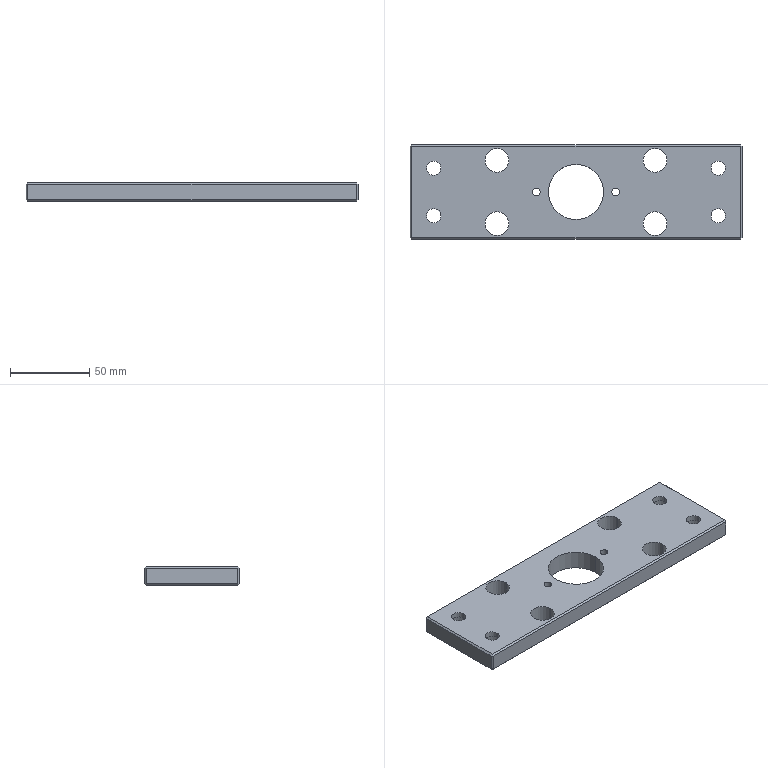Part | STEP file | 04-21 cylinder support bracket | 1 solid | 92 faces | box 210 x 60 x 12 mm | volume 122855 mm3 | cylinder 46 | plane 30 | cone 16 | commonest cylinder face diameters 2.5 x16 15 x16 9 x8 5 x4 35 x2